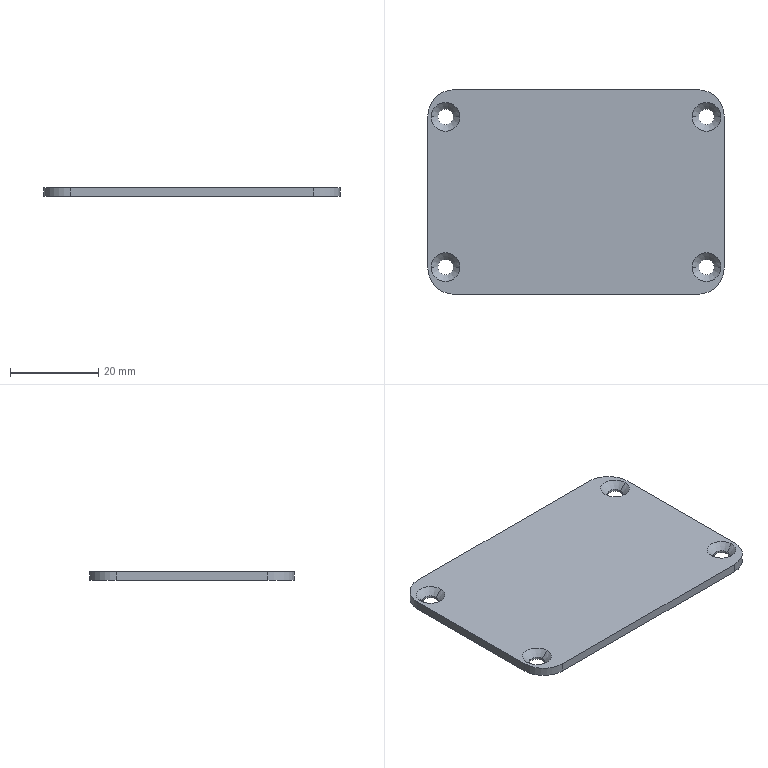Part | SolidWorks | features 3DProfileFeature 1, Extrusion 1, Fillet 1, HoleWzd 1, LPattern 1 | 1 solid | 26 faces | box 67 x 46.3 x 2 mm | volume 6002 mm3 | cylinder 12 | cone 8 | plane 6 | commonest cylinder face diameters 3.5 x8 12 x4
STEP:
#1=CARTESIAN_POINT('',(27.75,17.,0.5));
#2=VERTEX_POINT('',#1);
#3=CARTESIAN_POINT('',(31.25,17.,0.5));
#4=VERTEX_POINT('',#3);
#5=CARTESIAN_POINT('',(29.5,17.,0.5));
#6=DIRECTION('',(0.,0.,1.));
#7=DIRECTION('',(1.,0.,0.));
#8=AXIS2_PLACEMENT_3D('',#5,#6,#7);
#9=CIRCLE('',#8,1.75);
#10=EDGE_CURVE('',#2,#4,#9,.T.);
#11=ORIENTED_EDGE('',*,*,#10,.F.);
#12=CARTESIAN_POINT('',(26.25,17.,2.));
#13=VERTEX_POINT('',#12);
#14=CARTESIAN_POINT('',(26.25,17.,2.));
#15=DIRECTION('',(-0.7071,0.,0.7071));
#16=VECTOR('',#15,1000.);
#17=LINE('',#14,#16);
#18=EDGE_CURVE('',#2,#13,#17,.T.);
#19=ORIENTED_EDGE('',*,*,#18,.T.);
#20=CARTESIAN_POINT('',(32.75,17.,2.));
#21=VERTEX_POINT('',#20);
#22=CARTESIAN_POINT('',(29.5,17.,2.));
#23=DIRECTION('',(0.,0.,1.));
#24=DIRECTION('',(1.,0.,0.));
#25=AXIS2_PLACEMENT_3D('',#22,#23,#24);
#26=CIRCLE('',#25,3.25);
#27=EDGE_CURVE('',#13,#21,#26,.T.);
#28=ORIENTED_EDGE('',*,*,#27,.T.);
#29=CARTESIAN_POINT('',(32.75,17.,2.));
#30=DIRECTION('',(0.7071,0.,0.7071));
#31=VECTOR('',#30,1000.);
#32=LINE('',#29,#31);
#33=EDGE_CURVE('',#4,#21,#32,.T.);
#34=ORIENTED_EDGE('',*,*,#33,.F.);
#35=EDGE_LOOP('',(#11,#19,#28,#34));
#36=FACE_OUTER_BOUND('',#35,.T.);
#37=CARTESIAN_POINT('',(29.5,17.,2.));
#38=DIRECTION('',(0.,0.,1.));
#39=DIRECTION('',(1.,0.,0.));
#40=AXIS2_PLACEMENT_3D('',#37,#38,#39);
#41=CONICAL_SURFACE('',#40,3.25,0.7854);
#42=ADVANCED_FACE('',(#36),#41,.F.);
#43=CARTESIAN_POINT('',(27.75,17.,0.));
#44=VERTEX_POINT('',#43);
#45=CARTESIAN_POINT('',(31.25,17.,0.));
#46=VERTEX_POINT('',#45);
#47=CARTESIAN_POINT('',(29.5,17.,0.));
#48=DIRECTION('',(0.,0.,1.));
#49=DIRECTION('',(1.,0.,0.));
#50=AXIS2_PLACEMENT_3D('',#47,#48,#49);
#51=CIRCLE('',#50,1.75);
#52=EDGE_CURVE('',#44,#46,#51,.T.);
#53=ORIENTED_EDGE('',*,*,#52,.F.);
#54=CARTESIAN_POINT('',(27.75,17.,2.));
#55=DIRECTION('',(0.,0.,1.));
#56=VECTOR('',#55,1000.);
#57=LINE('',#54,#56);
#58=EDGE_CURVE('',#44,#2,#57,.T.);
#59=ORIENTED_EDGE('',*,*,#58,.T.);
#60=ORIENTED_EDGE('',*,*,#10,.T.);
#61=CARTESIAN_POINT('',(31.25,17.,2.));
#62=DIRECTION('',(0.,0.,1.));
#63=VECTOR('',#62,1000.);
#64=LINE('',#61,#63);
#65=EDGE_CURVE('',#46,#4,#64,.T.);
#66=ORIENTED_EDGE('',*,*,#65,.F.);
#67=EDGE_LOOP('',(#53,#59,#60,#66));
#68=FACE_OUTER_BOUND('',#67,.T.);
#69=CARTESIAN_POINT('',(29.5,17.,2.));
#70=DIRECTION('',(0.,0.,1.));
#71=DIRECTION('',(1.,0.,0.));
#72=AXIS2_PLACEMENT_3D('',#69,#70,#71);
#73=CYLINDRICAL_SURFACE('',#72,1.75);
#74=ADVANCED_FACE('',(#68),#73,.F.);
#75=CARTESIAN_POINT('',(-31.25,17.,0.5));
#76=VERTEX_POINT('',#75);
#77=CARTESIAN_POINT('',(-27.75,17.,0.5));
#78=VERTEX_POINT('',#77);
#79=CARTESIAN_POINT('',(-29.5,17.,0.5));
#80=DIRECTION('',(0.,0.,1.));
#81=DIRECTION('',(1.,0.,0.));
#82=AXIS2_PLACEMENT_3D('',#79,#80,#81);
#83=CIRCLE('',#82,1.75);
#84=EDGE_CURVE('',#76,#78,#83,.T.);
#85=ORIENTED_EDGE('',*,*,#84,.F.);
#86=CARTESIAN_POINT('',(-32.75,17.,2.));
#87=VERTEX_POINT('',#86);
#88=CARTESIAN_POINT('',(-32.75,17.,2.));
#89=DIRECTION('',(-0.7071,0.,0.7071));
#90=VECTOR('',#89,1000.);
#91=LINE('',#88,#90);
#92=EDGE_CURVE('',#76,#87,#91,.T.);
#93=ORIENTED_EDGE('',*,*,#92,.T.);
#94=CARTESIAN_POINT('',(-26.25,17.,2.));
#95=VERTEX_POINT('',#94);
#96=CARTESIAN_POINT('',(-29.5,17.,2.));
#97=DIRECTION('',(0.,0.,1.));
#98=DIRECTION('',(1.,0.,0.));
#99=AXIS2_PLACEMENT_3D('',#96,#97,#98);
#100=CIRCLE('',#99,3.25);
#101=EDGE_CURVE('',#87,#95,#100,.T.);
#102=ORIENTED_EDGE('',*,*,#101,.T.);
#103=CARTESIAN_POINT('',(-26.25,17.,2.));
#104=DIRECTION('',(0.7071,0.,0.7071));
#105=VECTOR('',#104,1000.);
#106=LINE('',#103,#105);
#107=EDGE_CURVE('',#78,#95,#106,.T.);
#108=ORIENTED_EDGE('',*,*,#107,.F.);
#109=EDGE_LOOP('',(#85,#93,#102,#108));
#110=FACE_OUTER_BOUND('',#109,.T.);
#111=CARTESIAN_POINT('',(-29.5,17.,2.));
#112=DIRECTION('',(0.,0.,1.));
#113=DIRECTION('',(1.,0.,0.));
#114=AXIS2_PLACEMENT_3D('',#111,#112,#113);
#115=CONICAL_SURFACE('',#114,3.25,0.7854);
#116=ADVANCED_FACE('',(#110),#115,.F.);
#117=CARTESIAN_POINT('',(-31.25,17.,0.));
#118=VERTEX_POINT('',#117);
#119=CARTESIAN_POINT('',(-27.75,17.,0.));
#120=VERTEX_POINT('',#119);
#121=CARTESIAN_POINT('',(-29.5,17.,0.));
#122=DIRECTION('',(0.,0.,1.));
#123=DIRECTION('',(1.,0.,0.));
#124=AXIS2_PLACEMENT_3D('',#121,#122,#123);
#125=CIRCLE('',#124,1.75);
#126=EDGE_CURVE('',#118,#120,#125,.T.);
#127=ORIENTED_EDGE('',*,*,#126,.F.);
#128=CARTESIAN_POINT('',(-31.25,17.,2.));
#129=DIRECTION('',(0.,0.,1.));
#130=VECTOR('',#129,1000.);
#131=LINE('',#128,#130);
#132=EDGE_CURVE('',#118,#76,#131,.T.);
#133=ORIENTED_EDGE('',*,*,#132,.T.);
#134=ORIENTED_EDGE('',*,*,#84,.T.);
#135=CARTESIAN_POINT('',(-27.75,17.,2.));
#136=DIRECTION('',(0.,0.,1.));
#137=VECTOR('',#136,1000.);
#138=LINE('',#135,#137);
#139=EDGE_CURVE('',#120,#78,#138,.T.);
#140=ORIENTED_EDGE('',*,*,#139,.F.);
#141=EDGE_LOOP('',(#127,#133,#134,#140));
#142=FACE_OUTER_BOUND('',#141,.T.);
#143=CARTESIAN_POINT('',(-29.5,17.,2.));
#144=DIRECTION('',(0.,0.,1.));
#145=DIRECTION('',(1.,0.,0.));
#146=AXIS2_PLACEMENT_3D('',#143,#144,#145);
#147=CYLINDRICAL_SURFACE('',#146,1.75);
#148=ADVANCED_FACE('',(#142),#147,.F.);
#149=CARTESIAN_POINT('',(27.75,-17.,0.5));
#150=VERTEX_POINT('',#149);
#151=CARTESIAN_POINT('',(31.25,-17.,0.5));
#152=VERTEX_POINT('',#151);
#153=CARTESIAN_POINT('',(29.5,-17.,0.5));
#154=DIRECTION('',(0.,0.,1.));
#155=DIRECTION('',(1.,0.,0.));
#156=AXIS2_PLACEMENT_3D('',#153,#154,#155);
#157=CIRCLE('',#156,1.75);
#158=EDGE_CURVE('',#150,#152,#157,.T.);
#159=ORIENTED_EDGE('',*,*,#158,.F.);
#160=CARTESIAN_POINT('',(26.25,-17.,2.));
#161=VERTEX_POINT('',#160);
#162=CARTESIAN_POINT('',(26.25,-17.,2.));
#163=DIRECTION('',(-0.7071,0.,0.7071));
#164=VECTOR('',#163,1000.);
#165=LINE('',#162,#164);
#166=EDGE_CURVE('',#150,#161,#165,.T.);
#167=ORIENTED_EDGE('',*,*,#166,.T.);
#168=CARTESIAN_POINT('',(32.75,-17.,2.));
#169=VERTEX_POINT('',#168);
#170=CARTESIAN_POINT('',(29.5,-17.,2.));
#171=DIRECTION('',(0.,0.,1.));
#172=DIRECTION('',(1.,0.,0.));
#173=AXIS2_PLACEMENT_3D('',#170,#171,#172);
#174=CIRCLE('',#173,3.25);
#175=EDGE_CURVE('',#161,#169,#174,.T.);
#176=ORIENTED_EDGE('',*,*,#175,.T.);
#177=CARTESIAN_POINT('',(32.75,-17.,2.));
#178=DIRECTION('',(0.7071,0.,0.7071));
#179=VECTOR('',#178,1000.);
#180=LINE('',#177,#179);
#181=EDGE_CURVE('',#152,#169,#180,.T.);
#182=ORIENTED_EDGE('',*,*,#181,.F.);
#183=EDGE_LOOP('',(#159,#167,#176,#182));
#184=FACE_OUTER_BOUND('',#183,.T.);
#185=CARTESIAN_POINT('',(29.5,-17.,2.));
#186=DIRECTION('',(0.,0.,1.));
#187=DIRECTION('',(1.,0.,0.));
#188=AXIS2_PLACEMENT_3D('',#185,#186,#187);
#189=CONICAL_SURFACE('',#188,3.25,0.7854);
#190=ADVANCED_FACE('',(#184),#189,.F.);
#191=CARTESIAN_POINT('',(27.75,-17.,0.));
#192=VERTEX_POINT('',#191);
#193=CARTESIAN_POINT('',(31.25,-17.,0.));
#194=VERTEX_POINT('',#193);
#195=CARTESIAN_POINT('',(29.5,-17.,0.));
#196=DIRECTION('',(0.,0.,1.));
#197=DIRECTION('',(1.,0.,0.));
#198=AXIS2_PLACEMENT_3D('',#195,#196,#197);
#199=CIRCLE('',#198,1.75);
#200=EDGE_CURVE('',#192,#194,#199,.T.);
#201=ORIENTED_EDGE('',*,*,#200,.F.);
#202=CARTESIAN_POINT('',(27.75,-17.,2.));
#203=DIRECTION('',(0.,0.,1.));
#204=VECTOR('',#203,1000.);
#205=LINE('',#202,#204);
#206=EDGE_CURVE('',#192,#150,#205,.T.);
#207=ORIENTED_EDGE('',*,*,#206,.T.);
#208=ORIENTED_EDGE('',*,*,#158,.T.);
#209=CARTESIAN_POINT('',(31.25,-17.,2.));
#210=DIRECTION('',(0.,0.,1.));
#211=VECTOR('',#210,1000.);
#212=LINE('',#209,#211);
#213=EDGE_CURVE('',#194,#152,#212,.T.);
#214=ORIENTED_EDGE('',*,*,#213,.F.);
#215=EDGE_LOOP('',(#201,#207,#208,#214));
#216=FACE_OUTER_BOUND('',#215,.T.);
#217=CARTESIAN_POINT('',(29.5,-17.,2.));
#218=DIRECTION('',(0.,0.,1.));
#219=DIRECTION('',(1.,0.,0.));
#220=AXIS2_PLACEMENT_3D('',#217,#218,#219);
#221=CYLINDRICAL_SURFACE('',#220,1.75);
#222=ADVANCED_FACE('',(#216),#221,.F.);
#223=CARTESIAN_POINT('',(-31.25,-17.,0.5));
#224=VERTEX_POINT('',#223);
#225=CARTESIAN_POINT('',(-27.75,-17.,0.5));
#226=VERTEX_POINT('',#225);
#227=CARTESIAN_POINT('',(-29.5,-17.,0.5));
#228=DIRECTION('',(0.,0.,1.));
#229=DIRECTION('',(1.,0.,0.));
#230=AXIS2_PLACEMENT_3D('',#227,#228,#229);
#231=CIRCLE('',#230,1.75);
#232=EDGE_CURVE('',#224,#226,#231,.T.);
#233=ORIENTED_EDGE('',*,*,#232,.F.);
#234=CARTESIAN_POINT('',(-32.75,-17.,2.));
#235=VERTEX_POINT('',#234);
#236=CARTESIAN_POINT('',(-32.75,-17.,2.));
#237=DIRECTION('',(-0.7071,0.,0.7071));
#238=VECTOR('',#237,1000.);
#239=LINE('',#236,#238);
#240=EDGE_CURVE('',#224,#235,#239,.T.);
#241=ORIENTED_EDGE('',*,*,#240,.T.);
#242=CARTESIAN_POINT('',(-26.25,-17.,2.));
#243=VERTEX_POINT('',#242);
#244=CARTESIAN_POINT('',(-29.5,-17.,2.));
#245=DIRECTION('',(0.,0.,1.));
#246=DIRECTION('',(1.,0.,0.));
#247=AXIS2_PLACEMENT_3D('',#244,#245,#246);
#248=CIRCLE('',#247,3.25);
#249=EDGE_CURVE('',#235,#243,#248,.T.);
#250=ORIENTED_EDGE('',*,*,#249,.T.);
#251=CARTESIAN_POINT('',(-26.25,-17.,2.));
#252=DIRECTION('',(0.7071,0.,0.7071));
#253=VECTOR('',#252,1000.);
#254=LINE('',#251,#253);
#255=EDGE_CURVE('',#226,#243,#254,.T.);
#256=ORIENTED_EDGE('',*,*,#255,.F.);
#257=EDGE_LOOP('',(#233,#241,#250,#256));
#258=FACE_OUTER_BOUND('',#257,.T.);
#259=CARTESIAN_POINT('',(-29.5,-17.,2.));
#260=DIRECTION('',(0.,0.,1.));
#261=DIRECTION('',(1.,0.,0.));
#262=AXIS2_PLACEMENT_3D('',#259,#260,#261);
#263=CONICAL_SURFACE('',#262,3.25,0.7854);
#264=ADVANCED_FACE('',(#258),#263,.F.);
#265=CARTESIAN_POINT('',(-31.25,-17.,0.));
#266=VERTEX_POINT('',#265);
#267=CARTESIAN_POINT('',(-27.75,-17.,0.));
#268=VERTEX_POINT('',#267);
#269=CARTESIAN_POINT('',(-29.5,-17.,0.));
#270=DIRECTION('',(0.,0.,1.));
#271=DIRECTION('',(1.,0.,0.));
#272=AXIS2_PLACEMENT_3D('',#269,#270,#271);
#273=CIRCLE('',#272,1.75);
#274=EDGE_CURVE('',#266,#268,#273,.T.);
#275=ORIENTED_EDGE('',*,*,#274,.F.);
#276=CARTESIAN_POINT('',(-31.25,-17.,2.));
#277=DIRECTION('',(0.,0.,1.));
#278=VECTOR('',#277,1000.);
#279=LINE('',#276,#278);
#280=EDGE_CURVE('',#266,#224,#279,.T.);
#281=ORIENTED_EDGE('',*,*,#280,.T.);
#282=ORIENTED_EDGE('',*,*,#232,.T.);
#283=CARTESIAN_POINT('',(-27.75,-17.,2.));
#284=DIRECTION('',(0.,0.,1.));
#285=VECTOR('',#284,1000.);
#286=LINE('',#283,#285);
#287=EDGE_CURVE('',#268,#226,#286,.T.);
#288=ORIENTED_EDGE('',*,*,#287,.F.);
#289=EDGE_LOOP('',(#275,#281,#282,#288));
#290=FACE_OUTER_BOUND('',#289,.T.);
#291=CARTESIAN_POINT('',(-29.5,-17.,2.));
#292=DIRECTION('',(0.,0.,1.));
#293=DIRECTION('',(1.,0.,0.));
#294=AXIS2_PLACEMENT_3D('',#291,#292,#293);
#295=CYLINDRICAL_SURFACE('',#294,1.75);
#296=ADVANCED_FACE('',(#290),#295,.F.);
#297=CARTESIAN_POINT('',(-33.5,17.15,0.));
#298=VERTEX_POINT('',#297);
#299=CARTESIAN_POINT('',(-33.5,-17.15,0.));
#300=VERTEX_POINT('',#299);
#301=CARTESIAN_POINT('',(-33.5,23.15,0.));
#302=DIRECTION('',(0.,-1.,0.));
#303=VECTOR('',#302,1000.);
#304=LINE('',#301,#303);
#305=EDGE_CURVE('',#298,#300,#304,.T.);
#306=ORIENTED_EDGE('',*,*,#305,.T.);
#307=CARTESIAN_POINT('',(-33.5,-17.15,2.));
#308=VERTEX_POINT('',#307);
#309=CARTESIAN_POINT('',(-33.5,-17.15,2.));
#310=DIRECTION('',(0.,0.,1.));
#311=VECTOR('',#310,1000.);
#312=LINE('',#309,#311);
#313=EDGE_CURVE('',#300,#308,#312,.T.);
#314=ORIENTED_EDGE('',*,*,#313,.T.);
#315=CARTESIAN_POINT('',(-33.5,17.15,2.));
#316=VERTEX_POINT('',#315);
#317=CARTESIAN_POINT('',(-33.5,23.15,2.));
#318=DIRECTION('',(0.,-1.,0.));
#319=VECTOR('',#318,1000.);
#320=LINE('',#317,#319);
#321=EDGE_CURVE('',#316,#308,#320,.T.);
#322=ORIENTED_EDGE('',*,*,#321,.F.);
#323=CARTESIAN_POINT('',(-33.5,17.15,2.));
#324=DIRECTION('',(0.,0.,-1.));
#325=VECTOR('',#324,1000.);
#326=LINE('',#323,#325);
#327=EDGE_CURVE('',#316,#298,#326,.T.);
#328=ORIENTED_EDGE('',*,*,#327,.T.);
#329=EDGE_LOOP('',(#306,#314,#322,#328));
#330=FACE_OUTER_BOUND('',#329,.T.);
#331=CARTESIAN_POINT('',(-33.5,23.15,2.));
#332=DIRECTION('',(1.,0.,0.));
#333=DIRECTION('',(0.,0.,-1.));
#334=AXIS2_PLACEMENT_3D('',#331,#332,#333);
#335=PLANE('',#334);
#336=ADVANCED_FACE('',(#330),#335,.F.);
#337=CARTESIAN_POINT('',(-27.5,-23.15,2.));
#338=VERTEX_POINT('',#337);
#339=CARTESIAN_POINT('',(27.5,-23.15,2.));
#340=VERTEX_POINT('',#339);
#341=CARTESIAN_POINT('',(-33.5,-23.15,2.));
#342=DIRECTION('',(1.,0.,0.));
#343=VECTOR('',#342,1000.);
#344=LINE('',#341,#343);
#345=EDGE_CURVE('',#338,#340,#344,.T.);
#346=ORIENTED_EDGE('',*,*,#345,.F.);
#347=CARTESIAN_POINT('',(-27.5,-23.15,0.));
#348=VERTEX_POINT('',#347);
#349=CARTESIAN_POINT('',(-27.5,-23.15,2.));
#350=DIRECTION('',(0.,0.,-1.));
#351=VECTOR('',#350,1000.);
#352=LINE('',#349,#351);
#353=EDGE_CURVE('',#338,#348,#352,.T.);
#354=ORIENTED_EDGE('',*,*,#353,.T.);
#355=CARTESIAN_POINT('',(27.5,-23.15,0.));
#356=VERTEX_POINT('',#355);
#357=CARTESIAN_POINT('',(-33.5,-23.15,0.));
#358=DIRECTION('',(1.,0.,0.));
#359=VECTOR('',#358,1000.);
#360=LINE('',#357,#359);
#361=EDGE_CURVE('',#348,#356,#360,.T.);
#362=ORIENTED_EDGE('',*,*,#361,.T.);
#363=CARTESIAN_POINT('',(27.5,-23.15,2.));
#364=DIRECTION('',(0.,0.,1.));
#365=VECTOR('',#364,1000.);
#366=LINE('',#363,#365);
#367=EDGE_CURVE('',#356,#340,#366,.T.);
#368=ORIENTED_EDGE('',*,*,#367,.T.);
#369=EDGE_LOOP('',(#346,#354,#362,#368));
#370=FACE_OUTER_BOUND('',#369,.T.);
#371=CARTESIAN_POINT('',(-33.5,-23.15,2.));
#372=DIRECTION('',(0.,1.,0.));
#373=DIRECTION('',(0.,0.,1.));
#374=AXIS2_PLACEMENT_3D('',#371,#372,#373);
#375=PLANE('',#374);
#376=ADVANCED_FACE('',(#370),#375,.F.);
#377=CARTESIAN_POINT('',(33.5,-17.15,2.));
#378=VERTEX_POINT('',#377);
#379=CARTESIAN_POINT('',(33.5,17.15,2.));
#380=VERTEX_POINT('',#379);
#381=CARTESIAN_POINT('',(33.5,23.15,2.));
#382=DIRECTION('',(0.,1.,0.));
#383=VECTOR('',#382,1000.);
#384=LINE('',#381,#383);
#385=EDGE_CURVE('',#378,#380,#384,.T.);
#386=ORIENTED_EDGE('',*,*,#385,.F.);
#387=CARTESIAN_POINT('',(33.5,-17.15,0.));
#388=VERTEX_POINT('',#387);
#389=CARTESIAN_POINT('',(33.5,-17.15,2.));
#390=DIRECTION('',(0.,0.,-1.));
#391=VECTOR('',#390,1000.);
#392=LINE('',#389,#391);
#393=EDGE_CURVE('',#378,#388,#392,.T.);
#394=ORIENTED_EDGE('',*,*,#393,.T.);
#395=CARTESIAN_POINT('',(33.5,17.15,0.));
#396=VERTEX_POINT('',#395);
#397=CARTESIAN_POINT('',(33.5,23.15,0.));
#398=DIRECTION('',(0.,1.,0.));
#399=VECTOR('',#398,1000.);
#400=LINE('',#397,#399);
#401=EDGE_CURVE('',#388,#396,#400,.T.);
#402=ORIENTED_EDGE('',*,*,#401,.T.);
#403=CARTESIAN_POINT('',(33.5,17.15,2.));
#404=DIRECTION('',(0.,0.,1.));
#405=VECTOR('',#404,1000.);
#406=LINE('',#403,#405);
#407=EDGE_CURVE('',#396,#380,#406,.T.);
#408=ORIENTED_EDGE('',*,*,#407,.T.);
#409=EDGE_LOOP('',(#386,#394,#402,#408));
#410=FACE_OUTER_BOUND('',#409,.T.);
#411=CARTESIAN_POINT('',(33.5,23.15,2.));
#412=DIRECTION('',(-1.,0.,0.));
#413=DIRECTION('',(0.,0.,1.));
#414=AXIS2_PLACEMENT_3D('',#411,#412,#413);
#415=PLANE('',#414);
#416=ADVANCED_FACE('',(#410),#415,.F.);
#417=CARTESIAN_POINT('',(27.5,23.15,2.));
#418=VERTEX_POINT('',#417);
#419=CARTESIAN_POINT('',(-27.5,23.15,2.));
#420=VERTEX_POINT('',#419);
#421=CARTESIAN_POINT('',(-33.5,23.15,2.));
#422=DIRECTION('',(-1.,0.,0.));
#423=VECTOR('',#422,1000.);
#424=LINE('',#421,#423);
#425=EDGE_CURVE('',#418,#420,#424,.T.);
#426=ORIENTED_EDGE('',*,*,#425,.F.);
#427=CARTESIAN_POINT('',(27.5,23.15,0.));
#428=VERTEX_POINT('',#427);
#429=CARTESIAN_POINT('',(27.5,23.15,2.));
#430=DIRECTION('',(0.,0.,-1.));
#431=VECTOR('',#430,1000.);
#432=LINE('',#429,#431);
#433=EDGE_CURVE('',#418,#428,#432,.T.);
#434=ORIENTED_EDGE('',*,*,#433,.T.);
#435=CARTESIAN_POINT('',(-27.5,23.15,0.));
#436=VERTEX_POINT('',#435);
#437=CARTESIAN_POINT('',(-33.5,23.15,0.));
#438=DIRECTION('',(-1.,0.,0.));
#439=VECTOR('',#438,1000.);
#440=LINE('',#437,#439);
#441=EDGE_CURVE('',#428,#436,#440,.T.);
#442=ORIENTED_EDGE('',*,*,#441,.T.);
#443=CARTESIAN_POINT('',(-27.5,23.15,2.));
#444=DIRECTION('',(0.,0.,1.));
#445=VECTOR('',#444,1000.);
#446=LINE('',#443,#445);
#447=EDGE_CURVE('',#436,#420,#446,.T.);
#448=ORIENTED_EDGE('',*,*,#447,.T.);
#449=EDGE_LOOP('',(#426,#434,#442,#448));
#450=FACE_OUTER_BOUND('',#449,.T.);
#451=CARTESIAN_POINT('',(-33.5,23.15,2.));
#452=DIRECTION('',(0.,-1.,0.));
#453=DIRECTION('',(0.,0.,-1.));
#454=AXIS2_PLACEMENT_3D('',#451,#452,#453);
#455=PLANE('',#454);
#456=ADVANCED_FACE('',(#450),#455,.F.);
#457=CARTESIAN_POINT('',(29.5,17.,2.));
#458=DIRECTION('',(0.,0.,1.));
#459=DIRECTION('',(1.,0.,0.));
#460=AXIS2_PLACEMENT_3D('',#457,#458,#459);
#461=CIRCLE('',#460,3.25);
#462=EDGE_CURVE('',#21,#13,#461,.T.);
#463=ORIENTED_EDGE('',*,*,#462,.F.);
#464=ORIENTED_EDGE('',*,*,#27,.F.);
#465=EDGE_LOOP('',(#463,#464));
#466=FACE_BOUND('',#465,.T.);
#467=CARTESIAN_POINT('',(-29.5,17.,2.));
#468=DIRECTION('',(0.,0.,1.));
#469=DIRECTION('',(1.,0.,0.));
#470=AXIS2_PLACEMENT_3D('',#467,#468,#469);
#471=CIRCLE('',#470,3.25);
#472=EDGE_CURVE('',#95,#87,#471,.T.);
#473=ORIENTED_EDGE('',*,*,#472,.F.);
#474=ORIENTED_EDGE('',*,*,#101,.F.);
#475=EDGE_LOOP('',(#473,#474));
#476=FACE_BOUND('',#475,.T.);
#477=CARTESIAN_POINT('',(29.5,-17.,2.));
#478=DIRECTION('',(0.,0.,1.));
#479=DIRECTION('',(1.,0.,0.));
#480=AXIS2_PLACEMENT_3D('',#477,#478,#479);
#481=CIRCLE('',#480,3.25);
#482=EDGE_CURVE('',#169,#161,#481,.T.);
#483=ORIENTED_EDGE('',*,*,#482,.F.);
#484=ORIENTED_EDGE('',*,*,#175,.F.);
#485=EDGE_LOOP('',(#483,#484));
#486=FACE_BOUND('',#485,.T.);
#487=CARTESIAN_POINT('',(-29.5,-17.,2.));
#488=DIRECTION('',(0.,0.,1.));
#489=DIRECTION('',(1.,0.,0.));
#490=AXIS2_PLACEMENT_3D('',#487,#488,#489);
#491=CIRCLE('',#490,3.25);
#492=EDGE_CURVE('',#243,#235,#491,.T.);
#493=ORIENTED_EDGE('',*,*,#492,.F.);
#494=ORIENTED_EDGE('',*,*,#249,.F.);
#495=EDGE_LOOP('',(#493,#494));
#496=FACE_BOUND('',#495,.T.);
#497=ORIENTED_EDGE('',*,*,#321,.T.);
#498=CARTESIAN_POINT('',(-27.5,-17.15,2.));
#499=DIRECTION('',(0.,0.,1.));
#500=DIRECTION('',(1.,0.,0.));
#501=AXIS2_PLACEMENT_3D('',#498,#499,#500);
#502=CIRCLE('',#501,6.);
#503=EDGE_CURVE('',#308,#338,#502,.T.);
#504=ORIENTED_EDGE('',*,*,#503,.T.);
#505=ORIENTED_EDGE('',*,*,#345,.T.);
#506=CARTESIAN_POINT('',(27.5,-17.15,2.));
#507=DIRECTION('',(0.,0.,1.));
#508=DIRECTION('',(1.,0.,0.));
#509=AXIS2_PLACEMENT_3D('',#506,#507,#508);
#510=CIRCLE('',#509,6.);
#511=EDGE_CURVE('',#340,#378,#510,.T.);
#512=ORIENTED_EDGE('',*,*,#511,.T.);
#513=ORIENTED_EDGE('',*,*,#385,.T.);
#514=CARTESIAN_POINT('',(27.5,17.15,2.));
#515=DIRECTION('',(0.,0.,1.));
#516=DIRECTION('',(1.,0.,0.));
#517=AXIS2_PLACEMENT_3D('',#514,#515,#516);
#518=CIRCLE('',#517,6.);
#519=EDGE_CURVE('',#380,#418,#518,.T.);
#520=ORIENTED_EDGE('',*,*,#519,.T.);
#521=ORIENTED_EDGE('',*,*,#425,.T.);
#522=CARTESIAN_POINT('',(-27.5,17.15,2.));
#523=DIRECTION('',(0.,0.,1.));
#524=DIRECTION('',(1.,0.,0.));
#525=AXIS2_PLACEMENT_3D('',#522,#523,#524);
#526=CIRCLE('',#525,6.);
#527=EDGE_CURVE('',#420,#316,#526,.T.);
#528=ORIENTED_EDGE('',*,*,#527,.T.);
#529=EDGE_LOOP('',(#497,#504,#505,#512,#513,#520,#521,#528));
#530=FACE_OUTER_BOUND('',#529,.T.);
#531=CARTESIAN_POINT('',(-33.5,-23.15,2.));
#532=DIRECTION('',(0.,0.,1.));
#533=DIRECTION('',(1.,0.,0.));
#534=AXIS2_PLACEMENT_3D('',#531,#532,#533);
#535=PLANE('',#534);
#536=ADVANCED_FACE('',(#466,#476,#486,#496,#530),#535,.T.);
#537=CARTESIAN_POINT('',(29.5,17.,0.));
#538=DIRECTION('',(0.,0.,1.));
#539=DIRECTION('',(1.,0.,0.));
#540=AXIS2_PLACEMENT_3D('',#537,#538,#539);
#541=CIRCLE('',#540,1.75);
#542=EDGE_CURVE('',#46,#44,#541,.T.);
#543=ORIENTED_EDGE('',*,*,#542,.T.);
#544=ORIENTED_EDGE('',*,*,#52,.T.);
#545=EDGE_LOOP('',(#543,#544));
#546=FACE_BOUND('',#545,.T.);
#547=CARTESIAN_POINT('',(-29.5,17.,0.));
#548=DIRECTION('',(0.,0.,1.));
#549=DIRECTION('',(1.,0.,0.));
#550=AXIS2_PLACEMENT_3D('',#547,#548,#549);
#551=CIRCLE('',#550,1.75);
#552=EDGE_CURVE('',#120,#118,#551,.T.);
#553=ORIENTED_EDGE('',*,*,#552,.T.);
#554=ORIENTED_EDGE('',*,*,#126,.T.);
#555=EDGE_LOOP('',(#553,#554));
#556=FACE_BOUND('',#555,.T.);
#557=CARTESIAN_POINT('',(29.5,-17.,0.));
#558=DIRECTION('',(0.,0.,1.));
#559=DIRECTION('',(1.,0.,0.));
#560=AXIS2_PLACEMENT_3D('',#557,#558,#559);
#561=CIRCLE('',#560,1.75);
#562=EDGE_CURVE('',#194,#192,#561,.T.);
#563=ORIENTED_EDGE('',*,*,#562,.T.);
#564=ORIENTED_EDGE('',*,*,#200,.T.);
#565=EDGE_LOOP('',(#563,#564));
#566=FACE_BOUND('',#565,.T.);
#567=CARTESIAN_POINT('',(-29.5,-17.,0.));
#568=DIRECTION('',(0.,0.,1.));
#569=DIRECTION('',(1.,0.,0.));
#570=AXIS2_PLACEMENT_3D('',#567,#568,#569);
#571=CIRCLE('',#570,1.75);
#572=EDGE_CURVE('',#268,#266,#571,.T.);
#573=ORIENTED_EDGE('',*,*,#572,.T.);
#574=ORIENTED_EDGE('',*,*,#274,.T.);
#575=EDGE_LOOP('',(#573,#574));
#576=FACE_BOUND('',#575,.T.);
#577=ORIENTED_EDGE('',*,*,#361,.F.);
#578=CARTESIAN_POINT('',(-27.5,-17.15,0.));
#579=DIRECTION('',(0.,0.,-1.));
#580=DIRECTION('',(1.,0.,0.));
#581=AXIS2_PLACEMENT_3D('',#578,#579,#580);
#582=CIRCLE('',#581,6.);
#583=EDGE_CURVE('',#348,#300,#582,.T.);
#584=ORIENTED_EDGE('',*,*,#583,.T.);
#585=ORIENTED_EDGE('',*,*,#305,.F.);
#586=CARTESIAN_POINT('',(-27.5,17.15,0.));
#587=DIRECTION('',(0.,0.,-1.));
#588=DIRECTION('',(1.,0.,0.));
#589=AXIS2_PLACEMENT_3D('',#586,#587,#588);
#590=CIRCLE('',#589,6.);
#591=EDGE_CURVE('',#298,#436,#590,.T.);
#592=ORIENTED_EDGE('',*,*,#591,.T.);
#593=ORIENTED_EDGE('',*,*,#441,.F.);
#594=CARTESIAN_POINT('',(27.5,17.15,0.));
#595=DIRECTION('',(0.,0.,-1.));
#596=DIRECTION('',(1.,0.,0.));
#597=AXIS2_PLACEMENT_3D('',#594,#595,#596);
#598=CIRCLE('',#597,6.);
#599=EDGE_CURVE('',#428,#396,#598,.T.);
#600=ORIENTED_EDGE('',*,*,#599,.T.);
#601=ORIENTED_EDGE('',*,*,#401,.F.);
#602=CARTESIAN_POINT('',(27.5,-17.15,0.));
#603=DIRECTION('',(0.,0.,-1.));
#604=DIRECTION('',(1.,0.,0.));
#605=AXIS2_PLACEMENT_3D('',#602,#603,#604);
#606=CIRCLE('',#605,6.);
#607=EDGE_CURVE('',#388,#356,#606,.T.);
#608=ORIENTED_EDGE('',*,*,#607,.T.);
#609=EDGE_LOOP('',(#577,#584,#585,#592,#593,#600,#601,#608));
#610=FACE_OUTER_BOUND('',#609,.T.);
#611=CARTESIAN_POINT('',(-33.5,-23.15,0.));
#612=DIRECTION('',(0.,0.,1.));
#613=DIRECTION('',(1.,0.,0.));
#614=AXIS2_PLACEMENT_3D('',#611,#612,#613);
#615=PLANE('',#614);
#616=ADVANCED_FACE('',(#546,#556,#566,#576,#610),#615,.F.);
#617=ORIENTED_EDGE('',*,*,#503,.F.);
#618=ORIENTED_EDGE('',*,*,#313,.F.);
#619=ORIENTED_EDGE('',*,*,#583,.F.);
#620=ORIENTED_EDGE('',*,*,#353,.F.);
#621=EDGE_LOOP('',(#617,#618,#619,#620));
#622=FACE_OUTER_BOUND('',#621,.T.);
#623=CARTESIAN_POINT('',(-27.5,-17.15,2.));
#624=DIRECTION('',(0.,0.,-1.));
#625=DIRECTION('',(-1.,0.,0.));
#626=AXIS2_PLACEMENT_3D('',#623,#624,#625);
#627=CYLINDRICAL_SURFACE('',#626,6.);
#628=ADVANCED_FACE('',(#622),#627,.T.);
#629=ORIENTED_EDGE('',*,*,#511,.F.);
#630=ORIENTED_EDGE('',*,*,#367,.F.);
#631=ORIENTED_EDGE('',*,*,#607,.F.);
#632=ORIENTED_EDGE('',*,*,#393,.F.);
#633=EDGE_LOOP('',(#629,#630,#631,#632));
#634=FACE_OUTER_BOUND('',#633,.T.);
#635=CARTESIAN_POINT('',(27.5,-17.15,2.));
#636=DIRECTION('',(0.,0.,-1.));
#637=DIRECTION('',(-1.,0.,0.));
#638=AXIS2_PLACEMENT_3D('',#635,#636,#637);
#639=CYLINDRICAL_SURFACE('',#638,6.);
#640=ADVANCED_FACE('',(#634),#639,.T.);
#641=ORIENTED_EDGE('',*,*,#519,.F.);
#642=ORIENTED_EDGE('',*,*,#407,.F.);
#643=ORIENTED_EDGE('',*,*,#599,.F.);
#644=ORIENTED_EDGE('',*,*,#433,.F.);
#645=EDGE_LOOP('',(#641,#642,#643,#644));
#646=FACE_OUTER_BOUND('',#645,.T.);
#647=CARTESIAN_POINT('',(27.5,17.15,2.));
#648=DIRECTION('',(0.,0.,-1.));
#649=DIRECTION('',(-1.,0.,0.));
#650=AXIS2_PLACEMENT_3D('',#647,#648,#649);
#651=CYLINDRICAL_SURFACE('',#650,6.);
#652=ADVANCED_FACE('',(#646),#651,.T.);
#653=ORIENTED_EDGE('',*,*,#527,.F.);
#654=ORIENTED_EDGE('',*,*,#447,.F.);
#655=ORIENTED_EDGE('',*,*,#591,.F.);
#656=ORIENTED_EDGE('',*,*,#327,.F.);
#657=EDGE_LOOP('',(#653,#654,#655,#656));
#658=FACE_OUTER_BOUND('',#657,.T.);
#659=CARTESIAN_POINT('',(-27.5,17.15,2.));
#660=DIRECTION('',(0.,0.,-1.));
#661=DIRECTION('',(-1.,0.,0.));
#662=AXIS2_PLACEMENT_3D('',#659,#660,#661);
#663=CYLINDRICAL_SURFACE('',#662,6.);
#664=ADVANCED_FACE('',(#658),#663,.T.);
#665=ORIENTED_EDGE('',*,*,#280,.F.);
#666=ORIENTED_EDGE('',*,*,#572,.F.);
#667=ORIENTED_EDGE('',*,*,#287,.T.);
#668=CARTESIAN_POINT('',(-29.5,-17.,0.5));
#669=DIRECTION('',(0.,0.,1.));
#670=DIRECTION('',(1.,0.,0.));
#671=AXIS2_PLACEMENT_3D('',#668,#669,#670);
#672=CIRCLE('',#671,1.75);
#673=EDGE_CURVE('',#226,#224,#672,.T.);
#674=ORIENTED_EDGE('',*,*,#673,.T.);
#675=EDGE_LOOP('',(#665,#666,#667,#674));
#676=FACE_OUTER_BOUND('',#675,.T.);
#677=CARTESIAN_POINT('',(-29.5,-17.,2.));
#678=DIRECTION('',(0.,0.,1.));
#679=DIRECTION('',(1.,0.,0.));
#680=AXIS2_PLACEMENT_3D('',#677,#678,#679);
#681=CYLINDRICAL_SURFACE('',#680,1.75);
#682=ADVANCED_FACE('',(#676),#681,.F.);
#683=ORIENTED_EDGE('',*,*,#240,.F.);
#684=ORIENTED_EDGE('',*,*,#673,.F.);
#685=ORIENTED_EDGE('',*,*,#255,.T.);
#686=ORIENTED_EDGE('',*,*,#492,.T.);
#687=EDGE_LOOP('',(#683,#684,#685,#686));
#688=FACE_OUTER_BOUND('',#687,.T.);
#689=CARTESIAN_POINT('',(-29.5,-17.,2.));
#690=DIRECTION('',(0.,0.,1.));
#691=DIRECTION('',(1.,0.,0.));
#692=AXIS2_PLACEMENT_3D('',#689,#690,#691);
#693=CONICAL_SURFACE('',#692,3.25,0.7854);
#694=ADVANCED_FACE('',(#688),#693,.F.);
#695=ORIENTED_EDGE('',*,*,#206,.F.);
#696=ORIENTED_EDGE('',*,*,#562,.F.);
#697=ORIENTED_EDGE('',*,*,#213,.T.);
#698=CARTESIAN_POINT('',(29.5,-17.,0.5));
#699=DIRECTION('',(0.,0.,1.));
#700=DIRECTION('',(1.,0.,0.));
#701=AXIS2_PLACEMENT_3D('',#698,#699,#700);
#702=CIRCLE('',#701,1.75);
#703=EDGE_CURVE('',#152,#150,#702,.T.);
#704=ORIENTED_EDGE('',*,*,#703,.T.);
#705=EDGE_LOOP('',(#695,#696,#697,#704));
#706=FACE_OUTER_BOUND('',#705,.T.);
#707=CARTESIAN_POINT('',(29.5,-17.,2.));
#708=DIRECTION('',(0.,0.,1.));
#709=DIRECTION('',(1.,0.,0.));
#710=AXIS2_PLACEMENT_3D('',#707,#708,#709);
#711=CYLINDRICAL_SURFACE('',#710,1.75);
#712=ADVANCED_FACE('',(#706),#711,.F.);
#713=ORIENTED_EDGE('',*,*,#166,.F.);
#714=ORIENTED_EDGE('',*,*,#703,.F.);
#715=ORIENTED_EDGE('',*,*,#181,.T.);
#716=ORIENTED_EDGE('',*,*,#482,.T.);
#717=EDGE_LOOP('',(#713,#714,#715,#716));
#718=FACE_OUTER_BOUND('',#717,.T.);
#719=CARTESIAN_POINT('',(29.5,-17.,2.));
#720=DIRECTION('',(0.,0.,1.));
#721=DIRECTION('',(1.,0.,0.));
#722=AXIS2_PLACEMENT_3D('',#719,#720,#721);
#723=CONICAL_SURFACE('',#722,3.25,0.7854);
#724=ADVANCED_FACE('',(#718),#723,.F.);
#725=ORIENTED_EDGE('',*,*,#132,.F.);
#726=ORIENTED_EDGE('',*,*,#552,.F.);
#727=ORIENTED_EDGE('',*,*,#139,.T.);
#728=CARTESIAN_POINT('',(-29.5,17.,0.5));
#729=DIRECTION('',(0.,0.,1.));
#730=DIRECTION('',(1.,0.,0.));
#731=AXIS2_PLACEMENT_3D('',#728,#729,#730);
#732=CIRCLE('',#731,1.75);
#733=EDGE_CURVE('',#78,#76,#732,.T.);
#734=ORIENTED_EDGE('',*,*,#733,.T.);
#735=EDGE_LOOP('',(#725,#726,#727,#734));
#736=FACE_OUTER_BOUND('',#735,.T.);
#737=CARTESIAN_POINT('',(-29.5,17.,2.));
#738=DIRECTION('',(0.,0.,1.));
#739=DIRECTION('',(1.,0.,0.));
#740=AXIS2_PLACEMENT_3D('',#737,#738,#739);
#741=CYLINDRICAL_SURFACE('',#740,1.75);
#742=ADVANCED_FACE('',(#736),#741,.F.);
#743=ORIENTED_EDGE('',*,*,#92,.F.);
#744=ORIENTED_EDGE('',*,*,#733,.F.);
#745=ORIENTED_EDGE('',*,*,#107,.T.);
#746=ORIENTED_EDGE('',*,*,#472,.T.);
#747=EDGE_LOOP('',(#743,#744,#745,#746));
#748=FACE_OUTER_BOUND('',#747,.T.);
#749=CARTESIAN_POINT('',(-29.5,17.,2.));
#750=DIRECTION('',(0.,0.,1.));
#751=DIRECTION('',(1.,0.,0.));
#752=AXIS2_PLACEMENT_3D('',#749,#750,#751);
#753=CONICAL_SURFACE('',#752,3.25,0.7854);
#754=ADVANCED_FACE('',(#748),#753,.F.);
#755=ORIENTED_EDGE('',*,*,#58,.F.);
#756=ORIENTED_EDGE('',*,*,#542,.F.);
#757=ORIENTED_EDGE('',*,*,#65,.T.);
#758=CARTESIAN_POINT('',(29.5,17.,0.5));
#759=DIRECTION('',(0.,0.,1.));
#760=DIRECTION('',(1.,0.,0.));
#761=AXIS2_PLACEMENT_3D('',#758,#759,#760);
#762=CIRCLE('',#761,1.75);
#763=EDGE_CURVE('',#4,#2,#762,.T.);
#764=ORIENTED_EDGE('',*,*,#763,.T.);
#765=EDGE_LOOP('',(#755,#756,#757,#764));
#766=FACE_OUTER_BOUND('',#765,.T.);
#767=CARTESIAN_POINT('',(29.5,17.,2.));
#768=DIRECTION('',(0.,0.,1.));
#769=DIRECTION('',(1.,0.,0.));
#770=AXIS2_PLACEMENT_3D('',#767,#768,#769);
#771=CYLINDRICAL_SURFACE('',#770,1.75);
#772=ADVANCED_FACE('',(#766),#771,.F.);
#773=ORIENTED_EDGE('',*,*,#18,.F.);
#774=ORIENTED_EDGE('',*,*,#763,.F.);
#775=ORIENTED_EDGE('',*,*,#33,.T.);
#776=ORIENTED_EDGE('',*,*,#462,.T.);
#777=EDGE_LOOP('',(#773,#774,#775,#776));
#778=FACE_OUTER_BOUND('',#777,.T.);
#779=CARTESIAN_POINT('',(29.5,17.,2.));
#780=DIRECTION('',(0.,0.,1.));
#781=DIRECTION('',(1.,0.,0.));
#782=AXIS2_PLACEMENT_3D('',#779,#780,#781);
#783=CONICAL_SURFACE('',#782,3.25,0.7854);
#784=ADVANCED_FACE('',(#778),#783,.F.);
#785=CLOSED_SHELL('',(#42,#74,#116,#148,#190,#222,#264,#296,#336,#376,#416,#456,#536,#616,#628,#640,#652,#664,#682,#694,#712,#724,#742,#754,#772,#784));
#786=MANIFOLD_SOLID_BREP('',#785);
#787=CARTESIAN_POINT('',(0.,0.,0.));
#788=DIRECTION('',(0.,0.,1.));
#789=DIRECTION('',(1.,0.,0.));
#790=AXIS2_PLACEMENT_3D('',#787,#788,#789);
#791=(LENGTH_UNIT()NAMED_UNIT(*)SI_UNIT(.MILLI.,.METRE.));
#792=UNCERTAINTY_MEASURE_WITH_UNIT(LENGTH_MEASURE(0.00001),#791,'','');
#793=(NAMED_UNIT(*)PLANE_ANGLE_UNIT()SI_UNIT($,.RADIAN.));
#794=(NAMED_UNIT(*)SI_UNIT($,.STERADIAN.)SOLID_ANGLE_UNIT());
#795=(GEOMETRIC_REPRESENTATION_CONTEXT(3)GLOBAL_UNCERTAINTY_ASSIGNED_CONTEXT((#792))GLOBAL_UNIT_ASSIGNED_CONTEXT((#791,#793,#794))REPRESENTATION_CONTEXT('',''));
#796=ADVANCED_BREP_SHAPE_REPRESENTATION('',(#786,#790),#795);